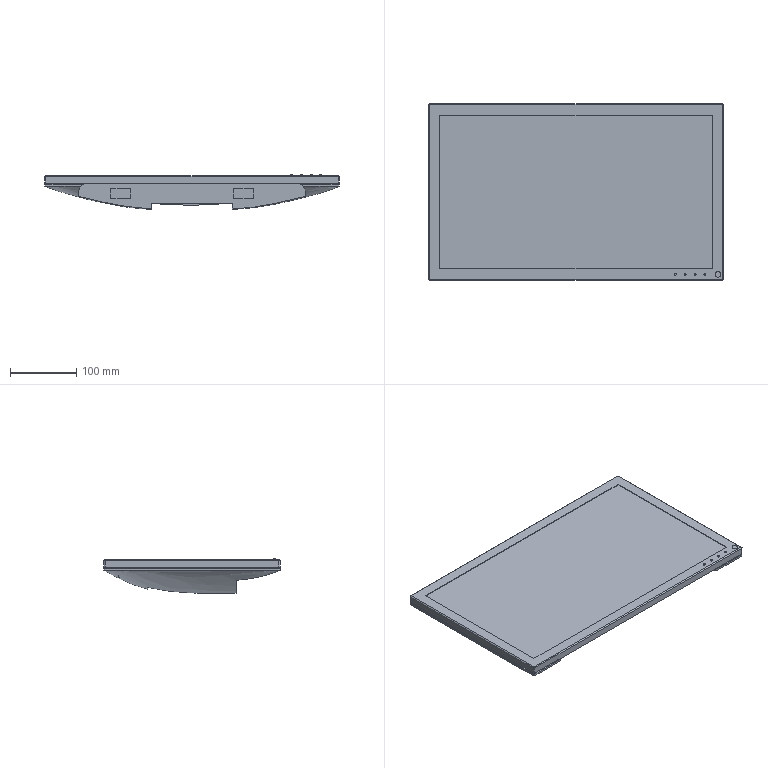Part | STEP file | E1916H Dell LCD monitor-ddde3r | 1 solid | 99 faces | box 445.5 x 266 x 52.76 mm | volume 3312642 mm3 | plane 52 | cylinder 20 | spline 19 | cone 8 | commonest cylinder face diameters 3.3 x8 4 x8 8.5 x2 30 x2